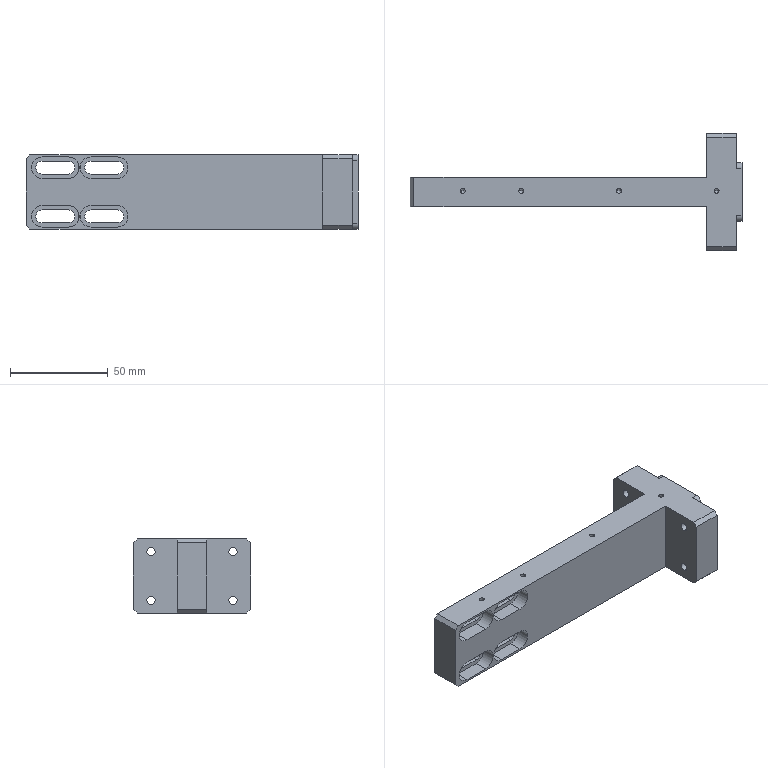Part | NX | features BREP 1 | 1 solid | 100 faces | box 170 x 60 x 38 mm | volume 112226 mm3 | cylinder 44 | plane 40 | cone 16 | commonest cylinder face diameters 2.5 x16 4.2 x8 6.6 x8 11 x8 6 x4